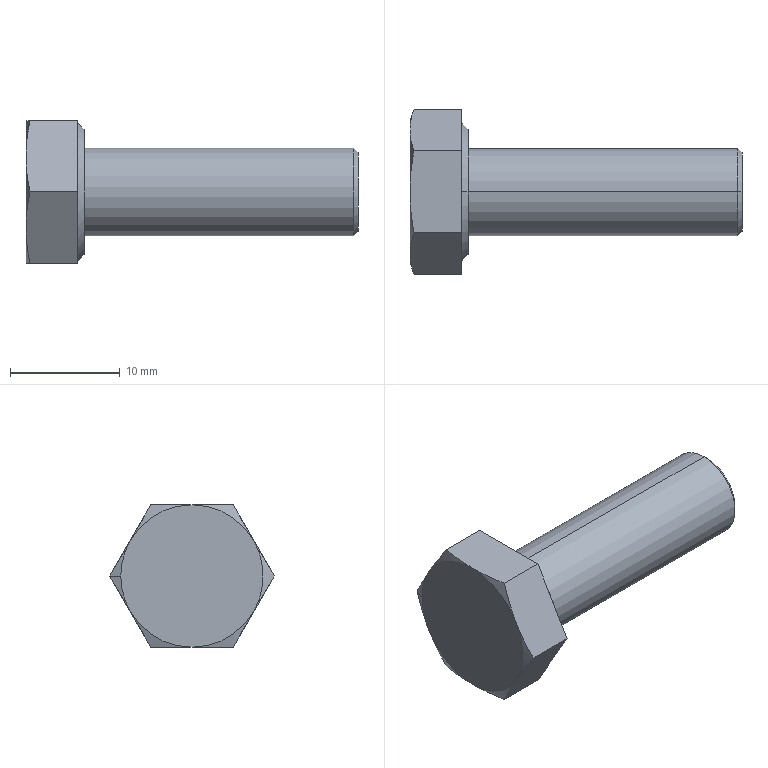Part | STEP file | hex head bolts-full thread grade c gb_GB_FASTENER_BOLT_HHBFTC M8X25-S | 1 solid | 23 faces | box 30.3 x 15.011 x 13 mm | volume 2010 mm3 | cone 11 | plane 10 | cylinder 2 | commonest cylinder face diameters 8 x2
STEP:
#1=CARTESIAN_POINT('',(29.9,0.,4.));
#2=VERTEX_POINT('',#1);
#3=CARTESIAN_POINT('',(29.9,0.,-4.));
#4=VERTEX_POINT('',#3);
#5=CARTESIAN_POINT('',(29.9,0.,0.));
#6=DIRECTION('',(-1.,0.,0.));
#7=DIRECTION('',(0.,0.,1.));
#8=AXIS2_PLACEMENT_3D('',#5,#6,#7);
#9=CIRCLE('',#8,4.);
#10=EDGE_CURVE('',#2,#4,#9,.T.);
#11=ORIENTED_EDGE('',*,*,#10,.T.);
#12=CARTESIAN_POINT('',(5.3,0.,-4.));
#13=VERTEX_POINT('',#12);
#14=CARTESIAN_POINT('',(30.3,0.,-4.));
#15=DIRECTION('',(-1.,0.,0.));
#16=VECTOR('',#15,1000.);
#17=LINE('',#14,#16);
#18=EDGE_CURVE('',#4,#13,#17,.T.);
#19=ORIENTED_EDGE('',*,*,#18,.T.);
#20=CARTESIAN_POINT('',(5.3,0.,4.));
#21=VERTEX_POINT('',#20);
#22=CARTESIAN_POINT('',(5.3,0.,0.));
#23=DIRECTION('',(1.,0.,0.));
#24=DIRECTION('',(0.,0.,1.));
#25=AXIS2_PLACEMENT_3D('',#22,#23,#24);
#26=CIRCLE('',#25,4.);
#27=EDGE_CURVE('',#13,#21,#26,.T.);
#28=ORIENTED_EDGE('',*,*,#27,.T.);
#29=CARTESIAN_POINT('',(30.3,0.,4.));
#30=DIRECTION('',(-1.,0.,0.));
#31=VECTOR('',#30,1000.);
#32=LINE('',#29,#31);
#33=EDGE_CURVE('',#2,#21,#32,.T.);
#34=ORIENTED_EDGE('',*,*,#33,.F.);
#35=EDGE_LOOP('',(#11,#19,#28,#34));
#36=FACE_OUTER_BOUND('',#35,.T.);
#37=CARTESIAN_POINT('',(30.3,0.,0.));
#38=DIRECTION('',(-1.,0.,0.));
#39=DIRECTION('',(0.,0.,1.));
#40=AXIS2_PLACEMENT_3D('',#37,#38,#39);
#41=CYLINDRICAL_SURFACE('',#40,4.);
#42=ADVANCED_FACE('',(#36),#41,.T.);
#43=CARTESIAN_POINT('',(30.3,0.,3.6));
#44=VERTEX_POINT('',#43);
#45=CARTESIAN_POINT('',(30.3,0.,-3.6));
#46=VERTEX_POINT('',#45);
#47=CARTESIAN_POINT('',(30.3,0.,0.));
#48=DIRECTION('',(-1.,0.,0.));
#49=DIRECTION('',(0.,0.,1.));
#50=AXIS2_PLACEMENT_3D('',#47,#48,#49);
#51=CIRCLE('',#50,3.6);
#52=EDGE_CURVE('',#44,#46,#51,.T.);
#53=ORIENTED_EDGE('',*,*,#52,.T.);
#54=CARTESIAN_POINT('',(29.9,0.,-4.));
#55=DIRECTION('',(-0.7071,0.,-0.7071));
#56=VECTOR('',#55,1000.);
#57=LINE('',#54,#56);
#58=EDGE_CURVE('',#46,#4,#57,.T.);
#59=ORIENTED_EDGE('',*,*,#58,.T.);
#60=ORIENTED_EDGE('',*,*,#10,.F.);
#61=CARTESIAN_POINT('',(29.9,0.,4.));
#62=DIRECTION('',(-0.7071,0.,0.7071));
#63=VECTOR('',#62,1000.);
#64=LINE('',#61,#63);
#65=EDGE_CURVE('',#44,#2,#64,.T.);
#66=ORIENTED_EDGE('',*,*,#65,.F.);
#67=EDGE_LOOP('',(#53,#59,#60,#66));
#68=FACE_OUTER_BOUND('',#67,.T.);
#69=CARTESIAN_POINT('',(29.9,0.,0.));
#70=DIRECTION('',(-1.,0.,0.));
#71=DIRECTION('',(0.,0.,1.));
#72=AXIS2_PLACEMENT_3D('',#69,#70,#71);
#73=CONICAL_SURFACE('',#72,4.,0.7854);
#74=ADVANCED_FACE('',(#68),#73,.T.);
#75=CARTESIAN_POINT('',(5.3,0.,5.735));
#76=VERTEX_POINT('',#75);
#77=CARTESIAN_POINT('',(5.3,0.,-5.735));
#78=VERTEX_POINT('',#77);
#79=CARTESIAN_POINT('',(5.3,0.,0.));
#80=DIRECTION('',(-1.,0.,0.));
#81=DIRECTION('',(0.,0.,1.));
#82=AXIS2_PLACEMENT_3D('',#79,#80,#81);
#83=CIRCLE('',#82,5.735);
#84=EDGE_CURVE('',#76,#78,#83,.T.);
#85=ORIENTED_EDGE('',*,*,#84,.T.);
#86=CARTESIAN_POINT('',(4.7,0.,-6.335));
#87=VERTEX_POINT('',#86);
#88=CARTESIAN_POINT('',(4.7,0.,-6.335));
#89=DIRECTION('',(-0.7071,0.,-0.7071));
#90=VECTOR('',#89,1000.);
#91=LINE('',#88,#90);
#92=EDGE_CURVE('',#78,#87,#91,.T.);
#93=ORIENTED_EDGE('',*,*,#92,.T.);
#94=CARTESIAN_POINT('',(4.7,0.,6.335));
#95=VERTEX_POINT('',#94);
#96=CARTESIAN_POINT('',(4.7,0.,0.));
#97=DIRECTION('',(1.,0.,0.));
#98=DIRECTION('',(0.,0.,1.));
#99=AXIS2_PLACEMENT_3D('',#96,#97,#98);
#100=CIRCLE('',#99,6.335);
#101=EDGE_CURVE('',#87,#95,#100,.T.);
#102=ORIENTED_EDGE('',*,*,#101,.T.);
#103=CARTESIAN_POINT('',(4.7,0.,6.335));
#104=DIRECTION('',(-0.7071,0.,0.7071));
#105=VECTOR('',#104,1000.);
#106=LINE('',#103,#105);
#107=EDGE_CURVE('',#76,#95,#106,.T.);
#108=ORIENTED_EDGE('',*,*,#107,.F.);
#109=EDGE_LOOP('',(#85,#93,#102,#108));
#110=FACE_OUTER_BOUND('',#109,.T.);
#111=CARTESIAN_POINT('',(4.7,0.,0.));
#112=DIRECTION('',(-1.,0.,0.));
#113=DIRECTION('',(0.,0.,1.));
#114=AXIS2_PLACEMENT_3D('',#111,#112,#113);
#115=CONICAL_SURFACE('',#114,6.335,0.7854);
#116=ADVANCED_FACE('',(#110),#115,.T.);
#117=CARTESIAN_POINT('',(0.,5.629,-3.25));
#118=VERTEX_POINT('',#117);
#119=CARTESIAN_POINT('',(0.,6.5,0.));
#120=VERTEX_POINT('',#119);
#121=CARTESIAN_POINT('',(0.,0.,0.));
#122=DIRECTION('',(1.,0.,0.));
#123=DIRECTION('',(0.,1.,0.));
#124=AXIS2_PLACEMENT_3D('',#121,#122,#123);
#125=CIRCLE('',#124,6.5);
#126=EDGE_CURVE('',#118,#120,#125,.T.);
#127=ORIENTED_EDGE('',*,*,#126,.T.);
#128=CARTESIAN_POINT('',(0.366,7.506,0.));
#129=VERTEX_POINT('',#128);
#130=CARTESIAN_POINT('',(0.3682,7.512,0.));
#131=DIRECTION('',(0.342,0.9397,0.));
#132=VECTOR('',#131,1000.);
#133=LINE('',#130,#132);
#134=EDGE_CURVE('',#120,#129,#133,.T.);
#135=ORIENTED_EDGE('',*,*,#134,.T.);
#136=CARTESIAN_POINT('',(0.366,7.506,0.));
#137=CARTESIAN_POINT('',(0.1402,6.885,-1.075));
#138=CARTESIAN_POINT('',(0.,6.261,-2.156));
#139=CARTESIAN_POINT('',(0.,5.629,-3.25));
#140=B_SPLINE_CURVE_WITH_KNOTS('',3,(#136,#137,#138,#139),.UNSPECIFIED.,.F.,.F.,(4,4),(0.,0.003771),.UNSPECIFIED.);
#141=EDGE_CURVE('',#129,#118,#140,.T.);
#142=ORIENTED_EDGE('',*,*,#141,.T.);
#143=EDGE_LOOP('',(#127,#135,#142));
#144=FACE_OUTER_BOUND('',#143,.T.);
#145=CARTESIAN_POINT('',(0.3682,0.,0.));
#146=DIRECTION('',(1.,0.,0.));
#147=DIRECTION('',(0.,1.,0.));
#148=AXIS2_PLACEMENT_3D('',#145,#146,#147);
#149=CONICAL_SURFACE('',#148,7.512,1.222);
#150=ADVANCED_FACE('',(#144),#149,.T.);
#151=ORIENTED_EDGE('',*,*,#18,.F.);
#152=CARTESIAN_POINT('',(29.9,0.,0.));
#153=DIRECTION('',(-1.,0.,0.));
#154=DIRECTION('',(0.,0.,1.));
#155=AXIS2_PLACEMENT_3D('',#152,#153,#154);
#156=CIRCLE('',#155,4.);
#157=EDGE_CURVE('',#4,#2,#156,.T.);
#158=ORIENTED_EDGE('',*,*,#157,.T.);
#159=ORIENTED_EDGE('',*,*,#33,.T.);
#160=CARTESIAN_POINT('',(5.3,0.,0.));
#161=DIRECTION('',(1.,0.,0.));
#162=DIRECTION('',(0.,0.,1.));
#163=AXIS2_PLACEMENT_3D('',#160,#161,#162);
#164=CIRCLE('',#163,4.);
#165=EDGE_CURVE('',#21,#13,#164,.T.);
#166=ORIENTED_EDGE('',*,*,#165,.T.);
#167=EDGE_LOOP('',(#151,#158,#159,#166));
#168=FACE_OUTER_BOUND('',#167,.T.);
#169=CARTESIAN_POINT('',(30.3,0.,0.));
#170=DIRECTION('',(-1.,0.,0.));
#171=DIRECTION('',(0.,0.,1.));
#172=AXIS2_PLACEMENT_3D('',#169,#170,#171);
#173=CYLINDRICAL_SURFACE('',#172,4.);
#174=ADVANCED_FACE('',(#168),#173,.T.);
#175=ORIENTED_EDGE('',*,*,#165,.F.);
#176=ORIENTED_EDGE('',*,*,#27,.F.);
#177=EDGE_LOOP('',(#175,#176));
#178=FACE_BOUND('',#177,.T.);
#179=ORIENTED_EDGE('',*,*,#84,.F.);
#180=CARTESIAN_POINT('',(5.3,0.,0.));
#181=DIRECTION('',(-1.,0.,0.));
#182=DIRECTION('',(0.,0.,1.));
#183=AXIS2_PLACEMENT_3D('',#180,#181,#182);
#184=CIRCLE('',#183,5.735);
#185=EDGE_CURVE('',#78,#76,#184,.T.);
#186=ORIENTED_EDGE('',*,*,#185,.F.);
#187=EDGE_LOOP('',(#179,#186));
#188=FACE_OUTER_BOUND('',#187,.T.);
#189=CARTESIAN_POINT('',(5.3,0.,13.));
#190=DIRECTION('',(-1.,0.,0.));
#191=DIRECTION('',(0.,0.,1.));
#192=AXIS2_PLACEMENT_3D('',#189,#190,#191);
#193=PLANE('',#192);
#194=ADVANCED_FACE('',(#178,#188),#193,.F.);
#195=ORIENTED_EDGE('',*,*,#58,.F.);
#196=CARTESIAN_POINT('',(30.3,0.,0.));
#197=DIRECTION('',(-1.,0.,0.));
#198=DIRECTION('',(0.,0.,1.));
#199=AXIS2_PLACEMENT_3D('',#196,#197,#198);
#200=CIRCLE('',#199,3.6);
#201=EDGE_CURVE('',#46,#44,#200,.T.);
#202=ORIENTED_EDGE('',*,*,#201,.T.);
#203=ORIENTED_EDGE('',*,*,#65,.T.);
#204=ORIENTED_EDGE('',*,*,#157,.F.);
#205=EDGE_LOOP('',(#195,#202,#203,#204));
#206=FACE_OUTER_BOUND('',#205,.T.);
#207=CARTESIAN_POINT('',(29.9,0.,0.));
#208=DIRECTION('',(-1.,0.,0.));
#209=DIRECTION('',(0.,0.,1.));
#210=AXIS2_PLACEMENT_3D('',#207,#208,#209);
#211=CONICAL_SURFACE('',#210,4.,0.7854);
#212=ADVANCED_FACE('',(#206),#211,.T.);
#213=ORIENTED_EDGE('',*,*,#92,.F.);
#214=ORIENTED_EDGE('',*,*,#185,.T.);
#215=ORIENTED_EDGE('',*,*,#107,.T.);
#216=CARTESIAN_POINT('',(4.7,0.,0.));
#217=DIRECTION('',(1.,0.,0.));
#218=DIRECTION('',(0.,0.,1.));
#219=AXIS2_PLACEMENT_3D('',#216,#217,#218);
#220=CIRCLE('',#219,6.335);
#221=EDGE_CURVE('',#95,#87,#220,.T.);
#222=ORIENTED_EDGE('',*,*,#221,.T.);
#223=EDGE_LOOP('',(#213,#214,#215,#222));
#224=FACE_OUTER_BOUND('',#223,.T.);
#225=CARTESIAN_POINT('',(4.7,0.,0.));
#226=DIRECTION('',(-1.,0.,0.));
#227=DIRECTION('',(0.,0.,1.));
#228=AXIS2_PLACEMENT_3D('',#225,#226,#227);
#229=CONICAL_SURFACE('',#228,6.335,0.7854);
#230=ADVANCED_FACE('',(#224),#229,.T.);
#231=ORIENTED_EDGE('',*,*,#52,.F.);
#232=ORIENTED_EDGE('',*,*,#201,.F.);
#233=EDGE_LOOP('',(#231,#232));
#234=FACE_OUTER_BOUND('',#233,.T.);
#235=CARTESIAN_POINT('',(30.3,0.,0.));
#236=DIRECTION('',(1.,0.,0.));
#237=DIRECTION('',(0.,0.,-1.));
#238=AXIS2_PLACEMENT_3D('',#235,#236,#237);
#239=PLANE('',#238);
#240=ADVANCED_FACE('',(#234),#239,.T.);
#241=CARTESIAN_POINT('',(4.7,7.506,0.));
#242=VERTEX_POINT('',#241);
#243=CARTESIAN_POINT('',(4.7,3.753,6.5));
#244=VERTEX_POINT('',#243);
#245=CARTESIAN_POINT('',(4.7,7.506,0.));
#246=DIRECTION('',(0.,-0.5,0.866));
#247=VECTOR('',#246,1000.);
#248=LINE('',#245,#247);
#249=EDGE_CURVE('',#242,#244,#248,.T.);
#250=ORIENTED_EDGE('',*,*,#249,.T.);
#251=CARTESIAN_POINT('',(4.7,-3.753,6.5));
#252=VERTEX_POINT('',#251);
#253=CARTESIAN_POINT('',(4.7,6.335,6.5));
#254=DIRECTION('',(0.,-1.,0.));
#255=VECTOR('',#254,1000.);
#256=LINE('',#253,#255);
#257=EDGE_CURVE('',#244,#252,#256,.T.);
#258=ORIENTED_EDGE('',*,*,#257,.T.);
#259=CARTESIAN_POINT('',(4.7,-7.506,0.));
#260=VERTEX_POINT('',#259);
#261=CARTESIAN_POINT('',(4.7,-3.753,6.5));
#262=DIRECTION('',(0.,-0.5,-0.866));
#263=VECTOR('',#262,1000.);
#264=LINE('',#261,#263);
#265=EDGE_CURVE('',#252,#260,#264,.T.);
#266=ORIENTED_EDGE('',*,*,#265,.T.);
#267=CARTESIAN_POINT('',(4.7,-3.753,-6.5));
#268=VERTEX_POINT('',#267);
#269=CARTESIAN_POINT('',(4.7,-7.506,0.));
#270=DIRECTION('',(0.,0.5,-0.866));
#271=VECTOR('',#270,1000.);
#272=LINE('',#269,#271);
#273=EDGE_CURVE('',#260,#268,#272,.T.);
#274=ORIENTED_EDGE('',*,*,#273,.T.);
#275=CARTESIAN_POINT('',(4.7,3.753,-6.5));
#276=VERTEX_POINT('',#275);
#277=CARTESIAN_POINT('',(4.7,6.335,-6.5));
#278=DIRECTION('',(0.,1.,0.));
#279=VECTOR('',#278,1000.);
#280=LINE('',#277,#279);
#281=EDGE_CURVE('',#268,#276,#280,.T.);
#282=ORIENTED_EDGE('',*,*,#281,.T.);
#283=CARTESIAN_POINT('',(4.7,3.753,-6.5));
#284=DIRECTION('',(0.,0.5,0.866));
#285=VECTOR('',#284,1000.);
#286=LINE('',#283,#285);
#287=EDGE_CURVE('',#276,#242,#286,.T.);
#288=ORIENTED_EDGE('',*,*,#287,.T.);
#289=EDGE_LOOP('',(#250,#258,#266,#274,#282,#288));
#290=FACE_OUTER_BOUND('',#289,.T.);
#291=ORIENTED_EDGE('',*,*,#221,.F.);
#292=ORIENTED_EDGE('',*,*,#101,.F.);
#293=EDGE_LOOP('',(#291,#292));
#294=FACE_BOUND('',#293,.T.);
#295=CARTESIAN_POINT('',(4.7,6.335,0.));
#296=DIRECTION('',(1.,0.,0.));
#297=DIRECTION('',(0.,0.,-1.));
#298=AXIS2_PLACEMENT_3D('',#295,#296,#297);
#299=PLANE('',#298);
#300=ADVANCED_FACE('',(#290,#294),#299,.T.);
#301=CARTESIAN_POINT('',(0.366,-3.753,6.5));
#302=VERTEX_POINT('',#301);
#303=CARTESIAN_POINT('',(5.3,-3.753,6.5));
#304=DIRECTION('',(-1.,0.,0.));
#305=VECTOR('',#304,1000.);
#306=LINE('',#303,#305);
#307=EDGE_CURVE('',#252,#302,#306,.T.);
#308=ORIENTED_EDGE('',*,*,#307,.F.);
#309=ORIENTED_EDGE('',*,*,#257,.F.);
#310=CARTESIAN_POINT('',(0.366,3.753,6.5));
#311=VERTEX_POINT('',#310);
#312=CARTESIAN_POINT('',(5.3,3.753,6.5));
#313=DIRECTION('',(1.,0.,0.));
#314=VECTOR('',#313,1000.);
#315=LINE('',#312,#314);
#316=EDGE_CURVE('',#311,#244,#315,.T.);
#317=ORIENTED_EDGE('',*,*,#316,.F.);
#318=CARTESIAN_POINT('',(0.,0.,6.5));
#319=VERTEX_POINT('',#318);
#320=CARTESIAN_POINT('',(0.,0.,6.5));
#321=CARTESIAN_POINT('',(0.,1.263,6.5));
#322=CARTESIAN_POINT('',(0.1402,2.512,6.5));
#323=CARTESIAN_POINT('',(0.366,3.753,6.5));
#324=B_SPLINE_CURVE_WITH_KNOTS('',3,(#320,#321,#322,#323),.UNSPECIFIED.,.F.,.F.,(4,4),(0.,0.003771),.UNSPECIFIED.);
#325=EDGE_CURVE('',#319,#311,#324,.T.);
#326=ORIENTED_EDGE('',*,*,#325,.F.);
#327=CARTESIAN_POINT('',(0.366,-3.753,6.5));
#328=CARTESIAN_POINT('',(0.1402,-2.512,6.5));
#329=CARTESIAN_POINT('',(0.,-1.263,6.5));
#330=CARTESIAN_POINT('',(0.,0.,6.5));
#331=B_SPLINE_CURVE_WITH_KNOTS('',3,(#327,#328,#329,#330),.UNSPECIFIED.,.F.,.F.,(4,4),(0.,0.003771),.UNSPECIFIED.);
#332=EDGE_CURVE('',#302,#319,#331,.T.);
#333=ORIENTED_EDGE('',*,*,#332,.F.);
#334=EDGE_LOOP('',(#308,#309,#317,#326,#333));
#335=FACE_OUTER_BOUND('',#334,.T.);
#336=CARTESIAN_POINT('',(5.3,3.753,6.5));
#337=DIRECTION('',(0.,0.,-1.));
#338=DIRECTION('',(-1.,0.,0.));
#339=AXIS2_PLACEMENT_3D('',#336,#337,#338);
#340=PLANE('',#339);
#341=ADVANCED_FACE('',(#335),#340,.F.);
#342=ORIENTED_EDGE('',*,*,#316,.T.);
#343=ORIENTED_EDGE('',*,*,#249,.F.);
#344=CARTESIAN_POINT('',(5.3,7.506,0.));
#345=DIRECTION('',(1.,0.,0.));
#346=VECTOR('',#345,1000.);
#347=LINE('',#344,#346);
#348=EDGE_CURVE('',#129,#242,#347,.T.);
#349=ORIENTED_EDGE('',*,*,#348,.F.);
#350=CARTESIAN_POINT('',(0.,5.629,3.25));
#351=VERTEX_POINT('',#350);
#352=CARTESIAN_POINT('',(0.,5.629,3.25));
#353=CARTESIAN_POINT('',(0.,6.261,2.156));
#354=CARTESIAN_POINT('',(0.1402,6.885,1.075));
#355=CARTESIAN_POINT('',(0.366,7.506,0.));
#356=B_SPLINE_CURVE_WITH_KNOTS('',3,(#352,#353,#354,#355),.UNSPECIFIED.,.F.,.F.,(4,4),(0.,0.003771),.UNSPECIFIED.);
#357=EDGE_CURVE('',#351,#129,#356,.T.);
#358=ORIENTED_EDGE('',*,*,#357,.F.);
#359=CARTESIAN_POINT('',(0.366,3.753,6.5));
#360=CARTESIAN_POINT('',(0.1402,4.373,5.425));
#361=CARTESIAN_POINT('',(0.,4.998,4.344));
#362=CARTESIAN_POINT('',(0.,5.629,3.25));
#363=B_SPLINE_CURVE_WITH_KNOTS('',3,(#359,#360,#361,#362),.UNSPECIFIED.,.F.,.F.,(4,4),(0.,0.003771),.UNSPECIFIED.);
#364=EDGE_CURVE('',#311,#351,#363,.T.);
#365=ORIENTED_EDGE('',*,*,#364,.F.);
#366=EDGE_LOOP('',(#342,#343,#349,#358,#365));
#367=FACE_OUTER_BOUND('',#366,.T.);
#368=CARTESIAN_POINT('',(5.3,7.506,0.));
#369=DIRECTION('',(0.,-0.866,-0.5));
#370=DIRECTION('',(0.,0.5,-0.866));
#371=AXIS2_PLACEMENT_3D('',#368,#369,#370);
#372=PLANE('',#371);
#373=ADVANCED_FACE('',(#367),#372,.F.);
#374=ORIENTED_EDGE('',*,*,#348,.T.);
#375=ORIENTED_EDGE('',*,*,#287,.F.);
#376=CARTESIAN_POINT('',(0.366,3.753,-6.5));
#377=VERTEX_POINT('',#376);
#378=CARTESIAN_POINT('',(5.3,3.753,-6.5));
#379=DIRECTION('',(1.,0.,0.));
#380=VECTOR('',#379,1000.);
#381=LINE('',#378,#380);
#382=EDGE_CURVE('',#377,#276,#381,.T.);
#383=ORIENTED_EDGE('',*,*,#382,.F.);
#384=CARTESIAN_POINT('',(0.,5.629,-3.25));
#385=CARTESIAN_POINT('',(0.,4.998,-4.344));
#386=CARTESIAN_POINT('',(0.1402,4.373,-5.425));
#387=CARTESIAN_POINT('',(0.366,3.753,-6.5));
#388=B_SPLINE_CURVE_WITH_KNOTS('',3,(#384,#385,#386,#387),.UNSPECIFIED.,.F.,.F.,(4,4),(0.,0.003771),.UNSPECIFIED.);
#389=EDGE_CURVE('',#118,#377,#388,.T.);
#390=ORIENTED_EDGE('',*,*,#389,.F.);
#391=ORIENTED_EDGE('',*,*,#141,.F.);
#392=EDGE_LOOP('',(#374,#375,#383,#390,#391));
#393=FACE_OUTER_BOUND('',#392,.T.);
#394=CARTESIAN_POINT('',(5.3,3.753,-6.5));
#395=DIRECTION('',(0.,-0.866,0.5));
#396=DIRECTION('',(0.,-0.5,-0.866));
#397=AXIS2_PLACEMENT_3D('',#394,#395,#396);
#398=PLANE('',#397);
#399=ADVANCED_FACE('',(#393),#398,.F.);
#400=ORIENTED_EDGE('',*,*,#382,.T.);
#401=ORIENTED_EDGE('',*,*,#281,.F.);
#402=CARTESIAN_POINT('',(0.366,-3.753,-6.5));
#403=VERTEX_POINT('',#402);
#404=CARTESIAN_POINT('',(5.3,-3.753,-6.5));
#405=DIRECTION('',(1.,0.,0.));
#406=VECTOR('',#405,1000.);
#407=LINE('',#404,#406);
#408=EDGE_CURVE('',#403,#268,#407,.T.);
#409=ORIENTED_EDGE('',*,*,#408,.F.);
#410=CARTESIAN_POINT('',(0.,0.,-6.5));
#411=VERTEX_POINT('',#410);
#412=CARTESIAN_POINT('',(0.,0.,-6.5));
#413=CARTESIAN_POINT('',(0.,-1.263,-6.5));
#414=CARTESIAN_POINT('',(0.1402,-2.512,-6.5));
#415=CARTESIAN_POINT('',(0.366,-3.753,-6.5));
#416=B_SPLINE_CURVE_WITH_KNOTS('',3,(#412,#413,#414,#415),.UNSPECIFIED.,.F.,.F.,(4,4),(0.,0.003771),.UNSPECIFIED.);
#417=EDGE_CURVE('',#411,#403,#416,.T.);
#418=ORIENTED_EDGE('',*,*,#417,.F.);
#419=CARTESIAN_POINT('',(0.366,3.753,-6.5));
#420=CARTESIAN_POINT('',(0.1402,2.512,-6.5));
#421=CARTESIAN_POINT('',(0.,1.263,-6.5));
#422=CARTESIAN_POINT('',(0.,0.,-6.5));
#423=B_SPLINE_CURVE_WITH_KNOTS('',3,(#419,#420,#421,#422),.UNSPECIFIED.,.F.,.F.,(4,4),(0.,0.003771),.UNSPECIFIED.);
#424=EDGE_CURVE('',#377,#411,#423,.T.);
#425=ORIENTED_EDGE('',*,*,#424,.F.);
#426=EDGE_LOOP('',(#400,#401,#409,#418,#425));
#427=FACE_OUTER_BOUND('',#426,.T.);
#428=CARTESIAN_POINT('',(5.3,-3.753,-6.5));
#429=DIRECTION('',(0.,0.,1.));
#430=DIRECTION('',(0.,-1.,0.));
#431=AXIS2_PLACEMENT_3D('',#428,#429,#430);
#432=PLANE('',#431);
#433=ADVANCED_FACE('',(#427),#432,.F.);
#434=ORIENTED_EDGE('',*,*,#408,.T.);
#435=ORIENTED_EDGE('',*,*,#273,.F.);
#436=CARTESIAN_POINT('',(0.366,-7.506,0.));
#437=VERTEX_POINT('',#436);
#438=CARTESIAN_POINT('',(5.3,-7.506,0.));
#439=DIRECTION('',(1.,0.,0.));
#440=VECTOR('',#439,1000.);
#441=LINE('',#438,#440);
#442=EDGE_CURVE('',#437,#260,#441,.T.);
#443=ORIENTED_EDGE('',*,*,#442,.F.);
#444=CARTESIAN_POINT('',(0.,-5.629,-3.25));
#445=VERTEX_POINT('',#444);
#446=CARTESIAN_POINT('',(0.,-5.629,-3.25));
#447=CARTESIAN_POINT('',(0.,-6.261,-2.156));
#448=CARTESIAN_POINT('',(0.1402,-6.885,-1.075));
#449=CARTESIAN_POINT('',(0.366,-7.506,0.));
#450=B_SPLINE_CURVE_WITH_KNOTS('',3,(#446,#447,#448,#449),.UNSPECIFIED.,.F.,.F.,(4,4),(0.,0.003771),.UNSPECIFIED.);
#451=EDGE_CURVE('',#445,#437,#450,.T.);
#452=ORIENTED_EDGE('',*,*,#451,.F.);
#453=CARTESIAN_POINT('',(0.366,-3.753,-6.5));
#454=CARTESIAN_POINT('',(0.1402,-4.373,-5.425));
#455=CARTESIAN_POINT('',(0.,-4.998,-4.344));
#456=CARTESIAN_POINT('',(0.,-5.629,-3.25));
#457=B_SPLINE_CURVE_WITH_KNOTS('',3,(#453,#454,#455,#456),.UNSPECIFIED.,.F.,.F.,(4,4),(0.,0.003771),.UNSPECIFIED.);
#458=EDGE_CURVE('',#403,#445,#457,.T.);
#459=ORIENTED_EDGE('',*,*,#458,.F.);
#460=EDGE_LOOP('',(#434,#435,#443,#452,#459));
#461=FACE_OUTER_BOUND('',#460,.T.);
#462=CARTESIAN_POINT('',(5.3,-7.506,0.));
#463=DIRECTION('',(0.,0.866,0.5));
#464=DIRECTION('',(0.,-0.5,0.866));
#465=AXIS2_PLACEMENT_3D('',#462,#463,#464);
#466=PLANE('',#465);
#467=ADVANCED_FACE('',(#461),#466,.F.);
#468=ORIENTED_EDGE('',*,*,#442,.T.);
#469=ORIENTED_EDGE('',*,*,#265,.F.);
#470=ORIENTED_EDGE('',*,*,#307,.T.);
#471=CARTESIAN_POINT('',(0.,-5.629,3.25));
#472=VERTEX_POINT('',#471);
#473=CARTESIAN_POINT('',(0.,-5.629,3.25));
#474=CARTESIAN_POINT('',(0.,-4.998,4.344));
#475=CARTESIAN_POINT('',(0.1402,-4.373,5.425));
#476=CARTESIAN_POINT('',(0.366,-3.753,6.5));
#477=B_SPLINE_CURVE_WITH_KNOTS('',3,(#473,#474,#475,#476),.UNSPECIFIED.,.F.,.F.,(4,4),(0.,0.003771),.UNSPECIFIED.);
#478=EDGE_CURVE('',#472,#302,#477,.T.);
#479=ORIENTED_EDGE('',*,*,#478,.F.);
#480=CARTESIAN_POINT('',(0.366,-7.506,0.));
#481=CARTESIAN_POINT('',(0.1402,-6.885,1.075));
#482=CARTESIAN_POINT('',(0.,-6.261,2.156));
#483=CARTESIAN_POINT('',(0.,-5.629,3.25));
#484=B_SPLINE_CURVE_WITH_KNOTS('',3,(#480,#481,#482,#483),.UNSPECIFIED.,.F.,.F.,(4,4),(0.,0.003771),.UNSPECIFIED.);
#485=EDGE_CURVE('',#437,#472,#484,.T.);
#486=ORIENTED_EDGE('',*,*,#485,.F.);
#487=EDGE_LOOP('',(#468,#469,#470,#479,#486));
#488=FACE_OUTER_BOUND('',#487,.T.);
#489=CARTESIAN_POINT('',(5.3,-3.753,6.5));
#490=DIRECTION('',(0.,0.866,-0.5));
#491=DIRECTION('',(0.,0.5,0.866));
#492=AXIS2_PLACEMENT_3D('',#489,#490,#491);
#493=PLANE('',#492);
#494=ADVANCED_FACE('',(#488),#493,.F.);
#495=ORIENTED_EDGE('',*,*,#332,.T.);
#496=CARTESIAN_POINT('',(0.,0.,0.));
#497=DIRECTION('',(1.,0.,0.));
#498=DIRECTION('',(0.,1.,0.));
#499=AXIS2_PLACEMENT_3D('',#496,#497,#498);
#500=CIRCLE('',#499,6.5);
#501=EDGE_CURVE('',#319,#472,#500,.T.);
#502=ORIENTED_EDGE('',*,*,#501,.T.);
#503=ORIENTED_EDGE('',*,*,#478,.T.);
#504=EDGE_LOOP('',(#495,#502,#503));
#505=FACE_OUTER_BOUND('',#504,.T.);
#506=CARTESIAN_POINT('',(0.3682,0.,0.));
#507=DIRECTION('',(1.,0.,0.));
#508=DIRECTION('',(0.,1.,0.));
#509=AXIS2_PLACEMENT_3D('',#506,#507,#508);
#510=CONICAL_SURFACE('',#509,7.512,1.222);
#511=ADVANCED_FACE('',(#505),#510,.T.);
#512=CARTESIAN_POINT('',(0.,0.,0.));
#513=DIRECTION('',(1.,0.,0.));
#514=DIRECTION('',(0.,1.,0.));
#515=AXIS2_PLACEMENT_3D('',#512,#513,#514);
#516=CIRCLE('',#515,6.5);
#517=EDGE_CURVE('',#351,#319,#516,.T.);
#518=ORIENTED_EDGE('',*,*,#517,.T.);
#519=ORIENTED_EDGE('',*,*,#325,.T.);
#520=ORIENTED_EDGE('',*,*,#364,.T.);
#521=EDGE_LOOP('',(#518,#519,#520));
#522=FACE_OUTER_BOUND('',#521,.T.);
#523=CARTESIAN_POINT('',(0.3682,0.,0.));
#524=DIRECTION('',(1.,0.,0.));
#525=DIRECTION('',(0.,1.,0.));
#526=AXIS2_PLACEMENT_3D('',#523,#524,#525);
#527=CONICAL_SURFACE('',#526,7.512,1.222);
#528=ADVANCED_FACE('',(#522),#527,.T.);
#529=ORIENTED_EDGE('',*,*,#134,.F.);
#530=CARTESIAN_POINT('',(0.,0.,0.));
#531=DIRECTION('',(1.,0.,0.));
#532=DIRECTION('',(0.,1.,0.));
#533=AXIS2_PLACEMENT_3D('',#530,#531,#532);
#534=CIRCLE('',#533,6.5);
#535=EDGE_CURVE('',#120,#351,#534,.T.);
#536=ORIENTED_EDGE('',*,*,#535,.T.);
#537=ORIENTED_EDGE('',*,*,#357,.T.);
#538=EDGE_LOOP('',(#529,#536,#537));
#539=FACE_OUTER_BOUND('',#538,.T.);
#540=CARTESIAN_POINT('',(0.3682,0.,0.));
#541=DIRECTION('',(1.,0.,0.));
#542=DIRECTION('',(0.,1.,0.));
#543=AXIS2_PLACEMENT_3D('',#540,#541,#542);
#544=CONICAL_SURFACE('',#543,7.512,1.222);
#545=ADVANCED_FACE('',(#539),#544,.T.);
#546=CARTESIAN_POINT('',(0.,0.,0.));
#547=DIRECTION('',(1.,0.,0.));
#548=DIRECTION('',(0.,1.,0.));
#549=AXIS2_PLACEMENT_3D('',#546,#547,#548);
#550=CIRCLE('',#549,6.5);
#551=EDGE_CURVE('',#411,#118,#550,.T.);
#552=ORIENTED_EDGE('',*,*,#551,.T.);
#553=ORIENTED_EDGE('',*,*,#389,.T.);
#554=ORIENTED_EDGE('',*,*,#424,.T.);
#555=EDGE_LOOP('',(#552,#553,#554));
#556=FACE_OUTER_BOUND('',#555,.T.);
#557=CARTESIAN_POINT('',(0.3682,0.,0.));
#558=DIRECTION('',(1.,0.,0.));
#559=DIRECTION('',(0.,1.,0.));
#560=AXIS2_PLACEMENT_3D('',#557,#558,#559);
#561=CONICAL_SURFACE('',#560,7.512,1.222);
#562=ADVANCED_FACE('',(#556),#561,.T.);
#563=ORIENTED_EDGE('',*,*,#458,.T.);
#564=CARTESIAN_POINT('',(0.,0.,0.));
#565=DIRECTION('',(1.,0.,0.));
#566=DIRECTION('',(0.,1.,0.));
#567=AXIS2_PLACEMENT_3D('',#564,#565,#566);
#568=CIRCLE('',#567,6.5);
#569=EDGE_CURVE('',#445,#411,#568,.T.);
#570=ORIENTED_EDGE('',*,*,#569,.T.);
#571=ORIENTED_EDGE('',*,*,#417,.T.);
#572=EDGE_LOOP('',(#563,#570,#571));
#573=FACE_OUTER_BOUND('',#572,.T.);
#574=CARTESIAN_POINT('',(0.3682,0.,0.));
#575=DIRECTION('',(1.,0.,0.));
#576=DIRECTION('',(0.,1.,0.));
#577=AXIS2_PLACEMENT_3D('',#574,#575,#576);
#578=CONICAL_SURFACE('',#577,7.512,1.222);
#579=ADVANCED_FACE('',(#573),#578,.T.);
#580=ORIENTED_EDGE('',*,*,#485,.T.);
#581=CARTESIAN_POINT('',(0.,0.,0.));
#582=DIRECTION('',(1.,0.,0.));
#583=DIRECTION('',(0.,1.,0.));
#584=AXIS2_PLACEMENT_3D('',#581,#582,#583);
#585=CIRCLE('',#584,6.5);
#586=EDGE_CURVE('',#472,#445,#585,.T.);
#587=ORIENTED_EDGE('',*,*,#586,.T.);
#588=ORIENTED_EDGE('',*,*,#451,.T.);
#589=EDGE_LOOP('',(#580,#587,#588));
#590=FACE_OUTER_BOUND('',#589,.T.);
#591=CARTESIAN_POINT('',(0.3682,0.,0.));
#592=DIRECTION('',(1.,0.,0.));
#593=DIRECTION('',(0.,1.,0.));
#594=AXIS2_PLACEMENT_3D('',#591,#592,#593);
#595=CONICAL_SURFACE('',#594,7.512,1.222);
#596=ADVANCED_FACE('',(#590),#595,.T.);
#597=ORIENTED_EDGE('',*,*,#569,.F.);
#598=ORIENTED_EDGE('',*,*,#586,.F.);
#599=ORIENTED_EDGE('',*,*,#501,.F.);
#600=ORIENTED_EDGE('',*,*,#517,.F.);
#601=ORIENTED_EDGE('',*,*,#535,.F.);
#602=ORIENTED_EDGE('',*,*,#126,.F.);
#603=ORIENTED_EDGE('',*,*,#551,.F.);
#604=EDGE_LOOP('',(#597,#598,#599,#600,#601,#602,#603));
#605=FACE_OUTER_BOUND('',#604,.T.);
#606=CARTESIAN_POINT('',(0.,0.,13.));
#607=DIRECTION('',(-1.,0.,0.));
#608=DIRECTION('',(0.,0.,1.));
#609=AXIS2_PLACEMENT_3D('',#606,#607,#608);
#610=PLANE('',#609);
#611=ADVANCED_FACE('',(#605),#610,.T.);
#612=CLOSED_SHELL('',(#42,#74,#116,#150,#174,#194,#212,#230,#240,#300,#341,#373,#399,#433,#467,#494,#511,#528,#545,#562,#579,#596,#611));
#613=MANIFOLD_SOLID_BREP('',#612);
#614=CARTESIAN_POINT('',(0.,0.,0.));
#615=DIRECTION('',(0.,0.,1.));
#616=DIRECTION('',(1.,0.,0.));
#617=AXIS2_PLACEMENT_3D('',#614,#615,#616);
#618=(LENGTH_UNIT()NAMED_UNIT(*)SI_UNIT(.MILLI.,.METRE.));
#619=UNCERTAINTY_MEASURE_WITH_UNIT(LENGTH_MEASURE(0.00001),#618,'','');
#620=(NAMED_UNIT(*)PLANE_ANGLE_UNIT()SI_UNIT($,.RADIAN.));
#621=(NAMED_UNIT(*)SI_UNIT($,.STERADIAN.)SOLID_ANGLE_UNIT());
#622=(GEOMETRIC_REPRESENTATION_CONTEXT(3)GLOBAL_UNCERTAINTY_ASSIGNED_CONTEXT((#619))GLOBAL_UNIT_ASSIGNED_CONTEXT((#618,#620,#621))REPRESENTATION_CONTEXT('',''));
#623=ADVANCED_BREP_SHAPE_REPRESENTATION('',(#613,#617),#622);